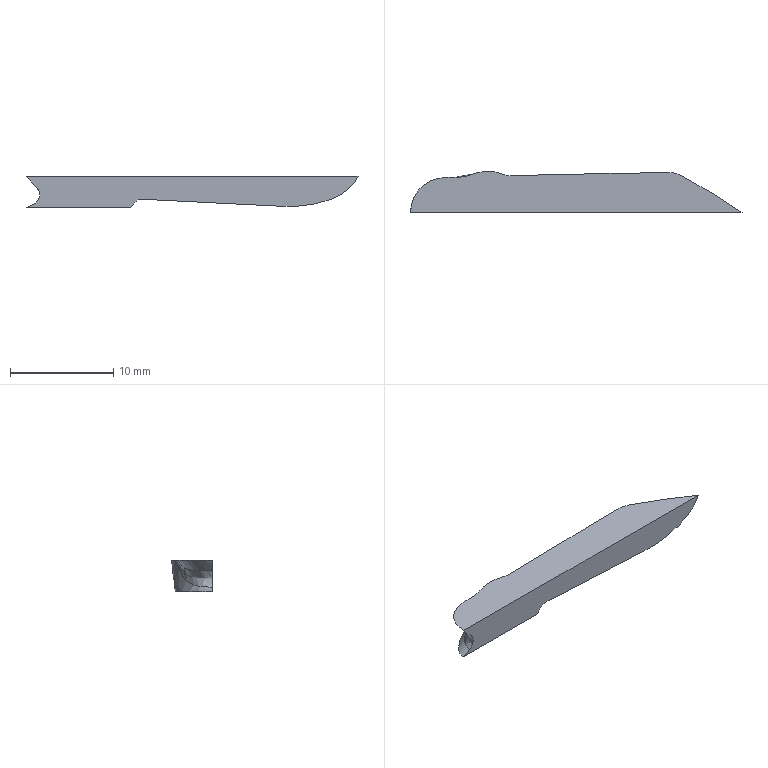Part | STEP file | solid 222 | 1 solid | 12 faces | box 32.172 x 3.969 x 3.297 mm | volume 218.611 mm3 | spline 6 | plane 3 | cylinder 2 | sphere 1 | commonest cylinder face diameters 8 x2